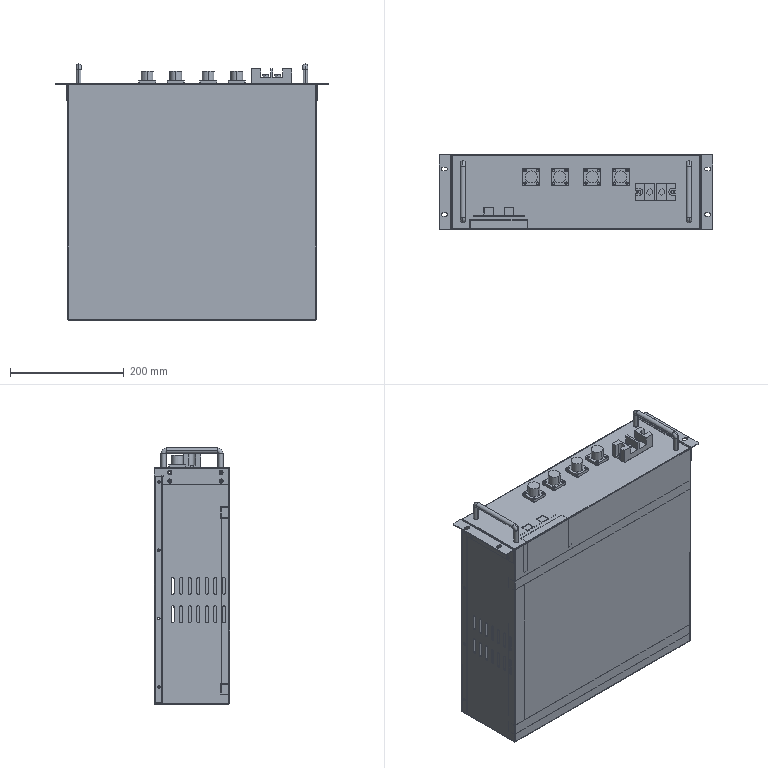Part | SolidWorks | features CompositeCurve 17, LocalLPattern 3, ReferencePattern 3 | 53 solids | 8245 faces | volume 2990736 mm3 | plane 3946 | cylinder 3354 | spline 822 | cone 108 | torus 13 | sphere 2 | commonest cylinder face diameters 0.305 x670 0.6 x231 4.5 x218 3.5 x140 0.381 x136 1 x129